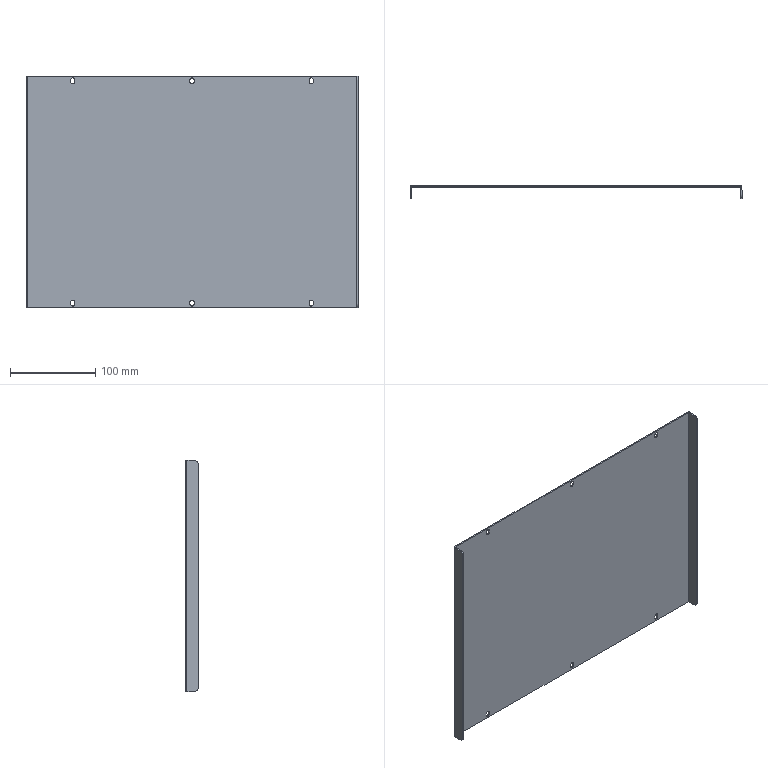Part | SolidWorks | features ICE 2, BreakCorner 1, EdgeFlange 1, FlatPattern 1, SMBaseFlange 1, SheetMetal 1 | 1 solid | 56 faces | box 390 x 15 x 272 mm | volume 169539 mm3 | plane 30 | cylinder 26 | commonest cylinder face diameters 5 x18 10 x4 0.2 x2 3.2 x2